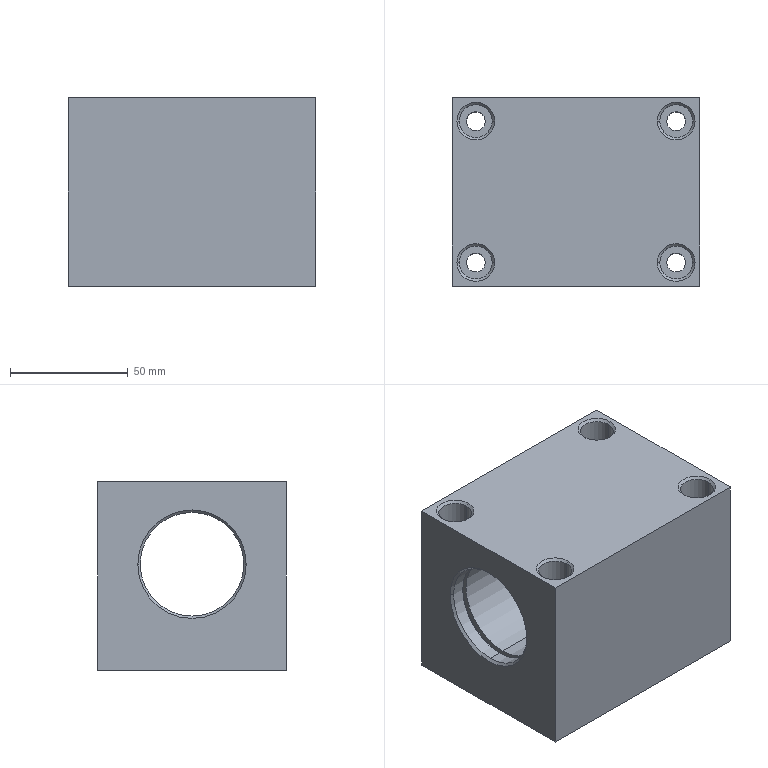Part | STEP file | Fixing block | 1 solid | 52 faces | box 105 x 80 x 80 mm | volume 486425 mm3 | cylinder 26 | plane 14 | cone 12 | commonest cylinder face diameters 8 x8 14 x8 44 x6 48.5 x4
STEP:
#1=CARTESIAN_POINT('',(-38.5,-30.,60.));
#2=VERTEX_POINT('',#1);
#3=CARTESIAN_POINT('',(-46.5,-30.,60.));
#4=VERTEX_POINT('',#3);
#5=CARTESIAN_POINT('',(-42.5,-30.,60.));
#6=DIRECTION('',(0.,0.,-1.));
#7=DIRECTION('',(-1.,0.,0.));
#8=AXIS2_PLACEMENT_3D('',#5,#6,#7);
#9=CIRCLE('',#8,4.);
#10=EDGE_CURVE('',#2,#4,#9,.T.);
#11=ORIENTED_EDGE('',*,*,#10,.F.);
#12=CARTESIAN_POINT('',(-38.5,-30.,0.));
#13=VERTEX_POINT('',#12);
#14=CARTESIAN_POINT('',(-38.5,-30.,80.));
#15=DIRECTION('',(0.,0.,-1.));
#16=VECTOR('',#15,1000.);
#17=LINE('',#14,#16);
#18=EDGE_CURVE('',#2,#13,#17,.T.);
#19=ORIENTED_EDGE('',*,*,#18,.T.);
#20=CARTESIAN_POINT('',(-46.5,-30.,0.));
#21=VERTEX_POINT('',#20);
#22=CARTESIAN_POINT('',(-42.5,-30.,0.));
#23=DIRECTION('',(0.,0.,-1.));
#24=DIRECTION('',(-1.,0.,0.));
#25=AXIS2_PLACEMENT_3D('',#22,#23,#24);
#26=CIRCLE('',#25,4.);
#27=EDGE_CURVE('',#13,#21,#26,.T.);
#28=ORIENTED_EDGE('',*,*,#27,.T.);
#29=CARTESIAN_POINT('',(-46.5,-30.,80.));
#30=DIRECTION('',(0.,0.,-1.));
#31=VECTOR('',#30,1000.);
#32=LINE('',#29,#31);
#33=EDGE_CURVE('',#4,#21,#32,.T.);
#34=ORIENTED_EDGE('',*,*,#33,.F.);
#35=EDGE_LOOP('',(#11,#19,#28,#34));
#36=FACE_OUTER_BOUND('',#35,.T.);
#37=CARTESIAN_POINT('',(-42.5,-30.,80.));
#38=DIRECTION('',(0.,0.,-1.));
#39=DIRECTION('',(-1.,0.,0.));
#40=AXIS2_PLACEMENT_3D('',#37,#38,#39);
#41=CYLINDRICAL_SURFACE('',#40,4.);
#42=ADVANCED_FACE('',(#36),#41,.F.);
#43=CARTESIAN_POINT('',(46.5,30.,60.));
#44=VERTEX_POINT('',#43);
#45=CARTESIAN_POINT('',(38.5,30.,60.));
#46=VERTEX_POINT('',#45);
#47=CARTESIAN_POINT('',(42.5,30.,60.));
#48=DIRECTION('',(0.,0.,-1.));
#49=DIRECTION('',(-1.,0.,0.));
#50=AXIS2_PLACEMENT_3D('',#47,#48,#49);
#51=CIRCLE('',#50,4.);
#52=EDGE_CURVE('',#44,#46,#51,.T.);
#53=ORIENTED_EDGE('',*,*,#52,.F.);
#54=CARTESIAN_POINT('',(46.5,30.,0.));
#55=VERTEX_POINT('',#54);
#56=CARTESIAN_POINT('',(46.5,30.,80.));
#57=DIRECTION('',(0.,0.,-1.));
#58=VECTOR('',#57,1000.);
#59=LINE('',#56,#58);
#60=EDGE_CURVE('',#44,#55,#59,.T.);
#61=ORIENTED_EDGE('',*,*,#60,.T.);
#62=CARTESIAN_POINT('',(38.5,30.,0.));
#63=VERTEX_POINT('',#62);
#64=CARTESIAN_POINT('',(42.5,30.,0.));
#65=DIRECTION('',(0.,0.,-1.));
#66=DIRECTION('',(-1.,0.,0.));
#67=AXIS2_PLACEMENT_3D('',#64,#65,#66);
#68=CIRCLE('',#67,4.);
#69=EDGE_CURVE('',#55,#63,#68,.T.);
#70=ORIENTED_EDGE('',*,*,#69,.T.);
#71=CARTESIAN_POINT('',(38.5,30.,80.));
#72=DIRECTION('',(0.,0.,-1.));
#73=VECTOR('',#72,1000.);
#74=LINE('',#71,#73);
#75=EDGE_CURVE('',#46,#63,#74,.T.);
#76=ORIENTED_EDGE('',*,*,#75,.F.);
#77=EDGE_LOOP('',(#53,#61,#70,#76));
#78=FACE_OUTER_BOUND('',#77,.T.);
#79=CARTESIAN_POINT('',(42.5,30.,80.));
#80=DIRECTION('',(0.,0.,-1.));
#81=DIRECTION('',(-1.,0.,0.));
#82=AXIS2_PLACEMENT_3D('',#79,#80,#81);
#83=CYLINDRICAL_SURFACE('',#82,4.);
#84=ADVANCED_FACE('',(#78),#83,.F.);
#85=CARTESIAN_POINT('',(-38.5,30.,60.));
#86=VERTEX_POINT('',#85);
#87=CARTESIAN_POINT('',(-46.5,30.,60.));
#88=VERTEX_POINT('',#87);
#89=CARTESIAN_POINT('',(-42.5,30.,60.));
#90=DIRECTION('',(0.,0.,-1.));
#91=DIRECTION('',(-1.,0.,0.));
#92=AXIS2_PLACEMENT_3D('',#89,#90,#91);
#93=CIRCLE('',#92,4.);
#94=EDGE_CURVE('',#86,#88,#93,.T.);
#95=ORIENTED_EDGE('',*,*,#94,.F.);
#96=CARTESIAN_POINT('',(-38.5,30.,0.));
#97=VERTEX_POINT('',#96);
#98=CARTESIAN_POINT('',(-38.5,30.,80.));
#99=DIRECTION('',(0.,0.,-1.));
#100=VECTOR('',#99,1000.);
#101=LINE('',#98,#100);
#102=EDGE_CURVE('',#86,#97,#101,.T.);
#103=ORIENTED_EDGE('',*,*,#102,.T.);
#104=CARTESIAN_POINT('',(-46.5,30.,0.));
#105=VERTEX_POINT('',#104);
#106=CARTESIAN_POINT('',(-42.5,30.,0.));
#107=DIRECTION('',(0.,0.,-1.));
#108=DIRECTION('',(-1.,0.,0.));
#109=AXIS2_PLACEMENT_3D('',#106,#107,#108);
#110=CIRCLE('',#109,4.);
#111=EDGE_CURVE('',#97,#105,#110,.T.);
#112=ORIENTED_EDGE('',*,*,#111,.T.);
#113=CARTESIAN_POINT('',(-46.5,30.,80.));
#114=DIRECTION('',(0.,0.,-1.));
#115=VECTOR('',#114,1000.);
#116=LINE('',#113,#115);
#117=EDGE_CURVE('',#88,#105,#116,.T.);
#118=ORIENTED_EDGE('',*,*,#117,.F.);
#119=EDGE_LOOP('',(#95,#103,#112,#118));
#120=FACE_OUTER_BOUND('',#119,.T.);
#121=CARTESIAN_POINT('',(-42.5,30.,80.));
#122=DIRECTION('',(0.,0.,-1.));
#123=DIRECTION('',(-1.,0.,0.));
#124=AXIS2_PLACEMENT_3D('',#121,#122,#123);
#125=CYLINDRICAL_SURFACE('',#124,4.);
#126=ADVANCED_FACE('',(#120),#125,.F.);
#127=CARTESIAN_POINT('',(46.5,-30.,60.));
#128=VERTEX_POINT('',#127);
#129=CARTESIAN_POINT('',(38.5,-30.,60.));
#130=VERTEX_POINT('',#129);
#131=CARTESIAN_POINT('',(42.5,-30.,60.));
#132=DIRECTION('',(0.,0.,-1.));
#133=DIRECTION('',(-1.,0.,0.));
#134=AXIS2_PLACEMENT_3D('',#131,#132,#133);
#135=CIRCLE('',#134,4.);
#136=EDGE_CURVE('',#128,#130,#135,.T.);
#137=ORIENTED_EDGE('',*,*,#136,.F.);
#138=CARTESIAN_POINT('',(46.5,-30.,0.));
#139=VERTEX_POINT('',#138);
#140=CARTESIAN_POINT('',(46.5,-30.,80.));
#141=DIRECTION('',(0.,0.,-1.));
#142=VECTOR('',#141,1000.);
#143=LINE('',#140,#142);
#144=EDGE_CURVE('',#128,#139,#143,.T.);
#145=ORIENTED_EDGE('',*,*,#144,.T.);
#146=CARTESIAN_POINT('',(38.5,-30.,0.));
#147=VERTEX_POINT('',#146);
#148=CARTESIAN_POINT('',(42.5,-30.,0.));
#149=DIRECTION('',(0.,0.,-1.));
#150=DIRECTION('',(-1.,0.,0.));
#151=AXIS2_PLACEMENT_3D('',#148,#149,#150);
#152=CIRCLE('',#151,4.);
#153=EDGE_CURVE('',#139,#147,#152,.T.);
#154=ORIENTED_EDGE('',*,*,#153,.T.);
#155=CARTESIAN_POINT('',(38.5,-30.,80.));
#156=DIRECTION('',(0.,0.,-1.));
#157=VECTOR('',#156,1000.);
#158=LINE('',#155,#157);
#159=EDGE_CURVE('',#130,#147,#158,.T.);
#160=ORIENTED_EDGE('',*,*,#159,.F.);
#161=EDGE_LOOP('',(#137,#145,#154,#160));
#162=FACE_OUTER_BOUND('',#161,.T.);
#163=CARTESIAN_POINT('',(42.5,-30.,80.));
#164=DIRECTION('',(0.,0.,-1.));
#165=DIRECTION('',(-1.,0.,0.));
#166=AXIS2_PLACEMENT_3D('',#163,#164,#165);
#167=CYLINDRICAL_SURFACE('',#166,4.);
#168=ADVANCED_FACE('',(#162),#167,.F.);
#169=CARTESIAN_POINT('',(-51.5,22.,45.));
#170=VERTEX_POINT('',#169);
#171=CARTESIAN_POINT('',(-51.5,0.,23.));
#172=VERTEX_POINT('',#171);
#173=CARTESIAN_POINT('',(-51.5,0.,45.));
#174=DIRECTION('',(-1.,0.,0.));
#175=DIRECTION('',(0.,0.,1.));
#176=AXIS2_PLACEMENT_3D('',#173,#174,#175);
#177=CIRCLE('',#176,22.);
#178=EDGE_CURVE('',#170,#172,#177,.T.);
#179=ORIENTED_EDGE('',*,*,#178,.F.);
#180=CARTESIAN_POINT('',(-52.5,23.,45.));
#181=VERTEX_POINT('',#180);
#182=CARTESIAN_POINT('',(-52.5,23.,45.));
#183=DIRECTION('',(-0.7071,0.7071,0.));
#184=VECTOR('',#183,1000.);
#185=LINE('',#182,#184);
#186=EDGE_CURVE('',#170,#181,#185,.T.);
#187=ORIENTED_EDGE('',*,*,#186,.T.);
#188=CARTESIAN_POINT('',(-52.5,-23.,45.));
#189=VERTEX_POINT('',#188);
#190=CARTESIAN_POINT('',(-52.5,0.,45.));
#191=DIRECTION('',(-1.,0.,0.));
#192=DIRECTION('',(0.,-1.,0.));
#193=AXIS2_PLACEMENT_3D('',#190,#191,#192);
#194=CIRCLE('',#193,23.);
#195=EDGE_CURVE('',#181,#189,#194,.T.);
#196=ORIENTED_EDGE('',*,*,#195,.T.);
#197=CARTESIAN_POINT('',(-51.5,-22.,45.));
#198=VERTEX_POINT('',#197);
#199=CARTESIAN_POINT('',(-52.5,-23.,45.));
#200=DIRECTION('',(-0.7071,-0.7071,0.));
#201=VECTOR('',#200,1000.);
#202=LINE('',#199,#201);
#203=EDGE_CURVE('',#198,#189,#202,.T.);
#204=ORIENTED_EDGE('',*,*,#203,.F.);
#205=CARTESIAN_POINT('',(-51.5,0.,45.));
#206=DIRECTION('',(-1.,0.,0.));
#207=DIRECTION('',(0.,0.,1.));
#208=AXIS2_PLACEMENT_3D('',#205,#206,#207);
#209=CIRCLE('',#208,22.);
#210=EDGE_CURVE('',#172,#198,#209,.T.);
#211=ORIENTED_EDGE('',*,*,#210,.F.);
#212=EDGE_LOOP('',(#179,#187,#196,#204,#211));
#213=FACE_OUTER_BOUND('',#212,.T.);
#214=CARTESIAN_POINT('',(-52.5,0.,45.));
#215=DIRECTION('',(-1.,0.,0.));
#216=DIRECTION('',(0.,-1.,0.));
#217=AXIS2_PLACEMENT_3D('',#214,#215,#216);
#218=CONICAL_SURFACE('',#217,23.,0.7854);
#219=ADVANCED_FACE('',(#213),#218,.F.);
#220=CARTESIAN_POINT('',(-49.5,30.,79.));
#221=VERTEX_POINT('',#220);
#222=CARTESIAN_POINT('',(-35.5,30.,79.));
#223=VERTEX_POINT('',#222);
#224=CARTESIAN_POINT('',(-42.5,30.,79.));
#225=DIRECTION('',(0.,0.,1.));
#226=DIRECTION('',(1.,0.,0.));
#227=AXIS2_PLACEMENT_3D('',#224,#225,#226);
#228=CIRCLE('',#227,7.);
#229=EDGE_CURVE('',#221,#223,#228,.T.);
#230=ORIENTED_EDGE('',*,*,#229,.F.);
#231=CARTESIAN_POINT('',(-50.5,30.,80.));
#232=VERTEX_POINT('',#231);
#233=CARTESIAN_POINT('',(-50.5,30.,80.));
#234=DIRECTION('',(-0.7071,0.,0.7071));
#235=VECTOR('',#234,1000.);
#236=LINE('',#233,#235);
#237=EDGE_CURVE('',#221,#232,#236,.T.);
#238=ORIENTED_EDGE('',*,*,#237,.T.);
#239=CARTESIAN_POINT('',(-34.5,30.,80.));
#240=VERTEX_POINT('',#239);
#241=CARTESIAN_POINT('',(-42.5,30.,80.));
#242=DIRECTION('',(0.,0.,-1.));
#243=DIRECTION('',(1.,0.,0.));
#244=AXIS2_PLACEMENT_3D('',#241,#242,#243);
#245=CIRCLE('',#244,8.);
#246=EDGE_CURVE('',#240,#232,#245,.T.);
#247=ORIENTED_EDGE('',*,*,#246,.F.);
#248=CARTESIAN_POINT('',(-34.5,30.,80.));
#249=DIRECTION('',(0.7071,0.,0.7071));
#250=VECTOR('',#249,1000.);
#251=LINE('',#248,#250);
#252=EDGE_CURVE('',#223,#240,#251,.T.);
#253=ORIENTED_EDGE('',*,*,#252,.F.);
#254=EDGE_LOOP('',(#230,#238,#247,#253));
#255=FACE_OUTER_BOUND('',#254,.T.);
#256=CARTESIAN_POINT('',(-42.5,30.,80.));
#257=DIRECTION('',(0.,0.,1.));
#258=DIRECTION('',(1.,0.,0.));
#259=AXIS2_PLACEMENT_3D('',#256,#257,#258);
#260=CONICAL_SURFACE('',#259,8.,0.7854);
#261=ADVANCED_FACE('',(#255),#260,.F.);
#262=CARTESIAN_POINT('',(-49.5,-30.,79.));
#263=VERTEX_POINT('',#262);
#264=CARTESIAN_POINT('',(-35.5,-30.,79.));
#265=VERTEX_POINT('',#264);
#266=CARTESIAN_POINT('',(-42.5,-30.,79.));
#267=DIRECTION('',(0.,0.,1.));
#268=DIRECTION('',(1.,0.,0.));
#269=AXIS2_PLACEMENT_3D('',#266,#267,#268);
#270=CIRCLE('',#269,7.);
#271=EDGE_CURVE('',#263,#265,#270,.T.);
#272=ORIENTED_EDGE('',*,*,#271,.F.);
#273=CARTESIAN_POINT('',(-50.5,-30.,80.));
#274=VERTEX_POINT('',#273);
#275=CARTESIAN_POINT('',(-50.5,-30.,80.));
#276=DIRECTION('',(-0.7071,0.,0.7071));
#277=VECTOR('',#276,1000.);
#278=LINE('',#275,#277);
#279=EDGE_CURVE('',#263,#274,#278,.T.);
#280=ORIENTED_EDGE('',*,*,#279,.T.);
#281=CARTESIAN_POINT('',(-34.5,-30.,80.));
#282=VERTEX_POINT('',#281);
#283=CARTESIAN_POINT('',(-42.5,-30.,80.));
#284=DIRECTION('',(0.,0.,-1.));
#285=DIRECTION('',(1.,0.,0.));
#286=AXIS2_PLACEMENT_3D('',#283,#284,#285);
#287=CIRCLE('',#286,8.);
#288=EDGE_CURVE('',#282,#274,#287,.T.);
#289=ORIENTED_EDGE('',*,*,#288,.F.);
#290=CARTESIAN_POINT('',(-34.5,-30.,80.));
#291=DIRECTION('',(0.7071,0.,0.7071));
#292=VECTOR('',#291,1000.);
#293=LINE('',#290,#292);
#294=EDGE_CURVE('',#265,#282,#293,.T.);
#295=ORIENTED_EDGE('',*,*,#294,.F.);
#296=EDGE_LOOP('',(#272,#280,#289,#295));
#297=FACE_OUTER_BOUND('',#296,.T.);
#298=CARTESIAN_POINT('',(-42.5,-30.,80.));
#299=DIRECTION('',(0.,0.,1.));
#300=DIRECTION('',(1.,0.,0.));
#301=AXIS2_PLACEMENT_3D('',#298,#299,#300);
#302=CONICAL_SURFACE('',#301,8.,0.7854);
#303=ADVANCED_FACE('',(#297),#302,.F.);
#304=CARTESIAN_POINT('',(35.5,30.,79.));
#305=VERTEX_POINT('',#304);
#306=CARTESIAN_POINT('',(49.5,30.,79.));
#307=VERTEX_POINT('',#306);
#308=CARTESIAN_POINT('',(42.5,30.,79.));
#309=DIRECTION('',(0.,0.,1.));
#310=DIRECTION('',(1.,0.,0.));
#311=AXIS2_PLACEMENT_3D('',#308,#309,#310);
#312=CIRCLE('',#311,7.);
#313=EDGE_CURVE('',#305,#307,#312,.T.);
#314=ORIENTED_EDGE('',*,*,#313,.F.);
#315=CARTESIAN_POINT('',(34.5,30.,80.));
#316=VERTEX_POINT('',#315);
#317=CARTESIAN_POINT('',(34.5,30.,80.));
#318=DIRECTION('',(-0.7071,0.,0.7071));
#319=VECTOR('',#318,1000.);
#320=LINE('',#317,#319);
#321=EDGE_CURVE('',#305,#316,#320,.T.);
#322=ORIENTED_EDGE('',*,*,#321,.T.);
#323=CARTESIAN_POINT('',(50.5,30.,80.));
#324=VERTEX_POINT('',#323);
#325=CARTESIAN_POINT('',(42.5,30.,80.));
#326=DIRECTION('',(0.,0.,-1.));
#327=DIRECTION('',(1.,0.,0.));
#328=AXIS2_PLACEMENT_3D('',#325,#326,#327);
#329=CIRCLE('',#328,8.);
#330=EDGE_CURVE('',#324,#316,#329,.T.);
#331=ORIENTED_EDGE('',*,*,#330,.F.);
#332=CARTESIAN_POINT('',(50.5,30.,80.));
#333=DIRECTION('',(0.7071,0.,0.7071));
#334=VECTOR('',#333,1000.);
#335=LINE('',#332,#334);
#336=EDGE_CURVE('',#307,#324,#335,.T.);
#337=ORIENTED_EDGE('',*,*,#336,.F.);
#338=EDGE_LOOP('',(#314,#322,#331,#337));
#339=FACE_OUTER_BOUND('',#338,.T.);
#340=CARTESIAN_POINT('',(42.5,30.,80.));
#341=DIRECTION('',(0.,0.,1.));
#342=DIRECTION('',(1.,0.,0.));
#343=AXIS2_PLACEMENT_3D('',#340,#341,#342);
#344=CONICAL_SURFACE('',#343,8.,0.7854);
#345=ADVANCED_FACE('',(#339),#344,.F.);
#346=CARTESIAN_POINT('',(35.5,-30.,79.));
#347=VERTEX_POINT('',#346);
#348=CARTESIAN_POINT('',(49.5,-30.,79.));
#349=VERTEX_POINT('',#348);
#350=CARTESIAN_POINT('',(42.5,-30.,79.));
#351=DIRECTION('',(0.,0.,1.));
#352=DIRECTION('',(1.,0.,0.));
#353=AXIS2_PLACEMENT_3D('',#350,#351,#352);
#354=CIRCLE('',#353,7.);
#355=EDGE_CURVE('',#347,#349,#354,.T.);
#356=ORIENTED_EDGE('',*,*,#355,.F.);
#357=CARTESIAN_POINT('',(34.5,-30.,80.));
#358=VERTEX_POINT('',#357);
#359=CARTESIAN_POINT('',(34.5,-30.,80.));
#360=DIRECTION('',(-0.7071,0.,0.7071));
#361=VECTOR('',#360,1000.);
#362=LINE('',#359,#361);
#363=EDGE_CURVE('',#347,#358,#362,.T.);
#364=ORIENTED_EDGE('',*,*,#363,.T.);
#365=CARTESIAN_POINT('',(50.5,-30.,80.));
#366=VERTEX_POINT('',#365);
#367=CARTESIAN_POINT('',(42.5,-30.,80.));
#368=DIRECTION('',(0.,0.,-1.));
#369=DIRECTION('',(1.,0.,0.));
#370=AXIS2_PLACEMENT_3D('',#367,#368,#369);
#371=CIRCLE('',#370,8.);
#372=EDGE_CURVE('',#366,#358,#371,.T.);
#373=ORIENTED_EDGE('',*,*,#372,.F.);
#374=CARTESIAN_POINT('',(50.5,-30.,80.));
#375=DIRECTION('',(0.7071,0.,0.7071));
#376=VECTOR('',#375,1000.);
#377=LINE('',#374,#376);
#378=EDGE_CURVE('',#349,#366,#377,.T.);
#379=ORIENTED_EDGE('',*,*,#378,.F.);
#380=EDGE_LOOP('',(#356,#364,#373,#379));
#381=FACE_OUTER_BOUND('',#380,.T.);
#382=CARTESIAN_POINT('',(42.5,-30.,80.));
#383=DIRECTION('',(0.,0.,1.));
#384=DIRECTION('',(1.,0.,0.));
#385=AXIS2_PLACEMENT_3D('',#382,#383,#384);
#386=CONICAL_SURFACE('',#385,8.,0.7854);
#387=ADVANCED_FACE('',(#381),#386,.F.);
#388=CARTESIAN_POINT('',(51.5,-22.,45.));
#389=VERTEX_POINT('',#388);
#390=CARTESIAN_POINT('',(51.5,0.,23.));
#391=VERTEX_POINT('',#390);
#392=CARTESIAN_POINT('',(51.5,0.,45.));
#393=DIRECTION('',(1.,0.,0.));
#394=DIRECTION('',(0.,0.,-1.));
#395=AXIS2_PLACEMENT_3D('',#392,#393,#394);
#396=CIRCLE('',#395,22.);
#397=EDGE_CURVE('',#389,#391,#396,.T.);
#398=ORIENTED_EDGE('',*,*,#397,.F.);
#399=CARTESIAN_POINT('',(52.5,-23.,45.));
#400=VERTEX_POINT('',#399);
#401=CARTESIAN_POINT('',(52.5,-23.,45.));
#402=DIRECTION('',(0.7071,-0.7071,0.));
#403=VECTOR('',#402,1000.);
#404=LINE('',#401,#403);
#405=EDGE_CURVE('',#389,#400,#404,.T.);
#406=ORIENTED_EDGE('',*,*,#405,.T.);
#407=CARTESIAN_POINT('',(52.5,23.,45.));
#408=VERTEX_POINT('',#407);
#409=CARTESIAN_POINT('',(52.5,0.,45.));
#410=DIRECTION('',(1.,0.,0.));
#411=DIRECTION('',(0.,1.,0.));
#412=AXIS2_PLACEMENT_3D('',#409,#410,#411);
#413=CIRCLE('',#412,23.);
#414=EDGE_CURVE('',#400,#408,#413,.T.);
#415=ORIENTED_EDGE('',*,*,#414,.T.);
#416=CARTESIAN_POINT('',(51.5,22.,45.));
#417=VERTEX_POINT('',#416);
#418=CARTESIAN_POINT('',(52.5,23.,45.));
#419=DIRECTION('',(0.7071,0.7071,0.));
#420=VECTOR('',#419,1000.);
#421=LINE('',#418,#420);
#422=EDGE_CURVE('',#417,#408,#421,.T.);
#423=ORIENTED_EDGE('',*,*,#422,.F.);
#424=CARTESIAN_POINT('',(51.5,0.,45.));
#425=DIRECTION('',(1.,0.,0.));
#426=DIRECTION('',(0.,0.,-1.));
#427=AXIS2_PLACEMENT_3D('',#424,#425,#426);
#428=CIRCLE('',#427,22.);
#429=EDGE_CURVE('',#391,#417,#428,.T.);
#430=ORIENTED_EDGE('',*,*,#429,.F.);
#431=EDGE_LOOP('',(#398,#406,#415,#423,#430));
#432=FACE_OUTER_BOUND('',#431,.T.);
#433=CARTESIAN_POINT('',(52.5,0.,45.));
#434=DIRECTION('',(1.,0.,0.));
#435=DIRECTION('',(0.,1.,0.));
#436=AXIS2_PLACEMENT_3D('',#433,#434,#435);
#437=CONICAL_SURFACE('',#436,23.,0.7854);
#438=ADVANCED_FACE('',(#432),#437,.F.);
#439=CARTESIAN_POINT('',(-46.,0.,23.));
#440=VERTEX_POINT('',#439);
#441=CARTESIAN_POINT('',(-46.,0.,67.));
#442=VERTEX_POINT('',#441);
#443=CARTESIAN_POINT('',(-46.,0.,45.));
#444=DIRECTION('',(-1.,0.,0.));
#445=DIRECTION('',(0.,0.,1.));
#446=AXIS2_PLACEMENT_3D('',#443,#444,#445);
#447=CIRCLE('',#446,22.);
#448=EDGE_CURVE('',#440,#442,#447,.T.);
#449=ORIENTED_EDGE('',*,*,#448,.F.);
#450=CARTESIAN_POINT('',(52.5,0.,23.));
#451=DIRECTION('',(-1.,0.,0.));
#452=VECTOR('',#451,1000.);
#453=LINE('',#450,#452);
#454=EDGE_CURVE('',#440,#172,#453,.T.);
#455=ORIENTED_EDGE('',*,*,#454,.T.);
#456=ORIENTED_EDGE('',*,*,#210,.T.);
#457=CARTESIAN_POINT('',(-51.5,0.,67.));
#458=VERTEX_POINT('',#457);
#459=CARTESIAN_POINT('',(-51.5,0.,45.));
#460=DIRECTION('',(-1.,0.,0.));
#461=DIRECTION('',(0.,0.,1.));
#462=AXIS2_PLACEMENT_3D('',#459,#460,#461);
#463=CIRCLE('',#462,22.);
#464=EDGE_CURVE('',#198,#458,#463,.T.);
#465=ORIENTED_EDGE('',*,*,#464,.T.);
#466=CARTESIAN_POINT('',(52.5,0.,67.));
#467=DIRECTION('',(-1.,0.,0.));
#468=VECTOR('',#467,1000.);
#469=LINE('',#466,#468);
#470=EDGE_CURVE('',#442,#458,#469,.T.);
#471=ORIENTED_EDGE('',*,*,#470,.F.);
#472=EDGE_LOOP('',(#449,#455,#456,#465,#471));
#473=FACE_OUTER_BOUND('',#472,.T.);
#474=CARTESIAN_POINT('',(52.5,0.,45.));
#475=DIRECTION('',(-1.,0.,0.));
#476=DIRECTION('',(0.,0.,1.));
#477=AXIS2_PLACEMENT_3D('',#474,#475,#476);
#478=CYLINDRICAL_SURFACE('',#477,22.);
#479=ADVANCED_FACE('',(#473),#478,.F.);
#480=CARTESIAN_POINT('',(-49.5,30.,60.));
#481=VERTEX_POINT('',#480);
#482=CARTESIAN_POINT('',(-35.5,30.,60.));
#483=VERTEX_POINT('',#482);
#484=CARTESIAN_POINT('',(-42.5,30.,60.));
#485=DIRECTION('',(0.,0.,1.));
#486=DIRECTION('',(1.,0.,0.));
#487=AXIS2_PLACEMENT_3D('',#484,#485,#486);
#488=CIRCLE('',#487,7.);
#489=EDGE_CURVE('',#481,#483,#488,.T.);
#490=ORIENTED_EDGE('',*,*,#489,.F.);
#491=CARTESIAN_POINT('',(-49.5,30.,60.));
#492=DIRECTION('',(0.,0.,1.));
#493=VECTOR('',#492,1000.);
#494=LINE('',#491,#493);
#495=EDGE_CURVE('',#481,#221,#494,.T.);
#496=ORIENTED_EDGE('',*,*,#495,.T.);
#497=ORIENTED_EDGE('',*,*,#229,.T.);
#498=CARTESIAN_POINT('',(-35.5,30.,60.));
#499=DIRECTION('',(0.,0.,1.));
#500=VECTOR('',#499,1000.);
#501=LINE('',#498,#500);
#502=EDGE_CURVE('',#483,#223,#501,.T.);
#503=ORIENTED_EDGE('',*,*,#502,.F.);
#504=EDGE_LOOP('',(#490,#496,#497,#503));
#505=FACE_OUTER_BOUND('',#504,.T.);
#506=CARTESIAN_POINT('',(-42.5,30.,60.));
#507=DIRECTION('',(0.,0.,1.));
#508=DIRECTION('',(1.,0.,0.));
#509=AXIS2_PLACEMENT_3D('',#506,#507,#508);
#510=CYLINDRICAL_SURFACE('',#509,7.);
#511=ADVANCED_FACE('',(#505),#510,.F.);
#512=CARTESIAN_POINT('',(-49.5,-30.,60.));
#513=VERTEX_POINT('',#512);
#514=CARTESIAN_POINT('',(-35.5,-30.,60.));
#515=VERTEX_POINT('',#514);
#516=CARTESIAN_POINT('',(-42.5,-30.,60.));
#517=DIRECTION('',(0.,0.,1.));
#518=DIRECTION('',(1.,0.,0.));
#519=AXIS2_PLACEMENT_3D('',#516,#517,#518);
#520=CIRCLE('',#519,7.);
#521=EDGE_CURVE('',#513,#515,#520,.T.);
#522=ORIENTED_EDGE('',*,*,#521,.F.);
#523=CARTESIAN_POINT('',(-49.5,-30.,60.));
#524=DIRECTION('',(0.,0.,1.));
#525=VECTOR('',#524,1000.);
#526=LINE('',#523,#525);
#527=EDGE_CURVE('',#513,#263,#526,.T.);
#528=ORIENTED_EDGE('',*,*,#527,.T.);
#529=ORIENTED_EDGE('',*,*,#271,.T.);
#530=CARTESIAN_POINT('',(-35.5,-30.,60.));
#531=DIRECTION('',(0.,0.,1.));
#532=VECTOR('',#531,1000.);
#533=LINE('',#530,#532);
#534=EDGE_CURVE('',#515,#265,#533,.T.);
#535=ORIENTED_EDGE('',*,*,#534,.F.);
#536=EDGE_LOOP('',(#522,#528,#529,#535));
#537=FACE_OUTER_BOUND('',#536,.T.);
#538=CARTESIAN_POINT('',(-42.5,-30.,60.));
#539=DIRECTION('',(0.,0.,1.));
#540=DIRECTION('',(1.,0.,0.));
#541=AXIS2_PLACEMENT_3D('',#538,#539,#540);
#542=CYLINDRICAL_SURFACE('',#541,7.);
#543=ADVANCED_FACE('',(#537),#542,.F.);
#544=CARTESIAN_POINT('',(35.5,30.,60.));
#545=VERTEX_POINT('',#544);
#546=CARTESIAN_POINT('',(49.5,30.,60.));
#547=VERTEX_POINT('',#546);
#548=CARTESIAN_POINT('',(42.5,30.,60.));
#549=DIRECTION('',(0.,0.,1.));
#550=DIRECTION('',(1.,0.,0.));
#551=AXIS2_PLACEMENT_3D('',#548,#549,#550);
#552=CIRCLE('',#551,7.);
#553=EDGE_CURVE('',#545,#547,#552,.T.);
#554=ORIENTED_EDGE('',*,*,#553,.F.);
#555=CARTESIAN_POINT('',(35.5,30.,60.));
#556=DIRECTION('',(0.,0.,1.));
#557=VECTOR('',#556,1000.);
#558=LINE('',#555,#557);
#559=EDGE_CURVE('',#545,#305,#558,.T.);
#560=ORIENTED_EDGE('',*,*,#559,.T.);
#561=ORIENTED_EDGE('',*,*,#313,.T.);
#562=CARTESIAN_POINT('',(49.5,30.,60.));
#563=DIRECTION('',(0.,0.,1.));
#564=VECTOR('',#563,1000.);
#565=LINE('',#562,#564);
#566=EDGE_CURVE('',#547,#307,#565,.T.);
#567=ORIENTED_EDGE('',*,*,#566,.F.);
#568=EDGE_LOOP('',(#554,#560,#561,#567));
#569=FACE_OUTER_BOUND('',#568,.T.);
#570=CARTESIAN_POINT('',(42.5,30.,60.));
#571=DIRECTION('',(0.,0.,1.));
#572=DIRECTION('',(1.,0.,0.));
#573=AXIS2_PLACEMENT_3D('',#570,#571,#572);
#574=CYLINDRICAL_SURFACE('',#573,7.);
#575=ADVANCED_FACE('',(#569),#574,.F.);
#576=CARTESIAN_POINT('',(35.5,-30.,60.));
#577=VERTEX_POINT('',#576);
#578=CARTESIAN_POINT('',(49.5,-30.,60.));
#579=VERTEX_POINT('',#578);
#580=CARTESIAN_POINT('',(42.5,-30.,60.));
#581=DIRECTION('',(0.,0.,1.));
#582=DIRECTION('',(1.,0.,0.));
#583=AXIS2_PLACEMENT_3D('',#580,#581,#582);
#584=CIRCLE('',#583,7.);
#585=EDGE_CURVE('',#577,#579,#584,.T.);
#586=ORIENTED_EDGE('',*,*,#585,.F.);
#587=CARTESIAN_POINT('',(35.5,-30.,60.));
#588=DIRECTION('',(0.,0.,1.));
#589=VECTOR('',#588,1000.);
#590=LINE('',#587,#589);
#591=EDGE_CURVE('',#577,#347,#590,.T.);
#592=ORIENTED_EDGE('',*,*,#591,.T.);
#593=ORIENTED_EDGE('',*,*,#355,.T.);
#594=CARTESIAN_POINT('',(49.5,-30.,60.));
#595=DIRECTION('',(0.,0.,1.));
#596=VECTOR('',#595,1000.);
#597=LINE('',#594,#596);
#598=EDGE_CURVE('',#579,#349,#597,.T.);
#599=ORIENTED_EDGE('',*,*,#598,.F.);
#600=EDGE_LOOP('',(#586,#592,#593,#599));
#601=FACE_OUTER_BOUND('',#600,.T.);
#602=CARTESIAN_POINT('',(42.5,-30.,60.));
#603=DIRECTION('',(0.,0.,1.));
#604=DIRECTION('',(1.,0.,0.));
#605=AXIS2_PLACEMENT_3D('',#602,#603,#604);
#606=CYLINDRICAL_SURFACE('',#605,7.);
#607=ADVANCED_FACE('',(#601),#606,.F.);
#608=CARTESIAN_POINT('',(51.5,0.,67.));
#609=VERTEX_POINT('',#608);
#610=CARTESIAN_POINT('',(51.5,0.,45.));
#611=DIRECTION('',(1.,0.,0.));
#612=DIRECTION('',(0.,0.,-1.));
#613=AXIS2_PLACEMENT_3D('',#610,#611,#612);
#614=CIRCLE('',#613,22.);
#615=EDGE_CURVE('',#609,#389,#614,.T.);
#616=ORIENTED_EDGE('',*,*,#615,.T.);
#617=ORIENTED_EDGE('',*,*,#397,.T.);
#618=CARTESIAN_POINT('',(46.,0.,23.));
#619=VERTEX_POINT('',#618);
#620=CARTESIAN_POINT('',(52.5,0.,23.));
#621=DIRECTION('',(-1.,0.,0.));
#622=VECTOR('',#621,1000.);
#623=LINE('',#620,#622);
#624=EDGE_CURVE('',#391,#619,#623,.T.);
#625=ORIENTED_EDGE('',*,*,#624,.T.);
#626=CARTESIAN_POINT('',(46.,0.,67.));
#627=VERTEX_POINT('',#626);
#628=CARTESIAN_POINT('',(46.,0.,45.));
#629=DIRECTION('',(1.,0.,0.));
#630=DIRECTION('',(0.,0.,1.));
#631=AXIS2_PLACEMENT_3D('',#628,#629,#630);
#632=CIRCLE('',#631,22.);
#633=EDGE_CURVE('',#627,#619,#632,.T.);
#634=ORIENTED_EDGE('',*,*,#633,.F.);
#635=CARTESIAN_POINT('',(52.5,0.,67.));
#636=DIRECTION('',(-1.,0.,0.));
#637=VECTOR('',#636,1000.);
#638=LINE('',#635,#637);
#639=EDGE_CURVE('',#609,#627,#638,.T.);
#640=ORIENTED_EDGE('',*,*,#639,.F.);
#641=EDGE_LOOP('',(#616,#617,#625,#634,#640));
#642=FACE_OUTER_BOUND('',#641,.T.);
#643=CARTESIAN_POINT('',(52.5,0.,45.));
#644=DIRECTION('',(-1.,0.,0.));
#645=DIRECTION('',(0.,0.,1.));
#646=AXIS2_PLACEMENT_3D('',#643,#644,#645);
#647=CYLINDRICAL_SURFACE('',#646,22.);
#648=ADVANCED_FACE('',(#642),#647,.F.);
#649=CARTESIAN_POINT('',(-46.,0.,69.25));
#650=VERTEX_POINT('',#649);
#651=CARTESIAN_POINT('',(-46.,0.,20.75));
#652=VERTEX_POINT('',#651);
#653=CARTESIAN_POINT('',(-46.,0.,45.));
#654=DIRECTION('',(1.,0.,0.));
#655=DIRECTION('',(0.,0.,-1.));
#656=AXIS2_PLACEMENT_3D('',#653,#654,#655);
#657=CIRCLE('',#656,24.25);
#658=EDGE_CURVE('',#650,#652,#657,.T.);
#659=ORIENTED_EDGE('',*,*,#658,.F.);
#660=CARTESIAN_POINT('',(-44.,0.,69.25));
#661=VERTEX_POINT('',#660);
#662=CARTESIAN_POINT('',(5.937,0.,69.25));
#663=DIRECTION('',(1.,0.,0.));
#664=VECTOR('',#663,1000.);
#665=LINE('',#662,#664);
#666=EDGE_CURVE('',#650,#661,#665,.T.);
#667=ORIENTED_EDGE('',*,*,#666,.T.);
#668=CARTESIAN_POINT('',(-44.,0.,20.75));
#669=VERTEX_POINT('',#668);
#670=CARTESIAN_POINT('',(-44.,0.,45.));
#671=DIRECTION('',(-1.,0.,0.));
#672=DIRECTION('',(0.,0.,-1.));
#673=AXIS2_PLACEMENT_3D('',#670,#671,#672);
#674=CIRCLE('',#673,24.25);
#675=EDGE_CURVE('',#669,#661,#674,.T.);
#676=ORIENTED_EDGE('',*,*,#675,.F.);
#677=CARTESIAN_POINT('',(5.937,0.,20.75));
#678=DIRECTION('',(1.,0.,0.));
#679=VECTOR('',#678,1000.);
#680=LINE('',#677,#679);
#681=EDGE_CURVE('',#652,#669,#680,.T.);
#682=ORIENTED_EDGE('',*,*,#681,.F.);
#683=EDGE_LOOP('',(#659,#667,#676,#682));
#684=FACE_OUTER_BOUND('',#683,.T.);
#685=CARTESIAN_POINT('',(5.937,0.,45.));
#686=DIRECTION('',(1.,0.,0.));
#687=DIRECTION('',(0.,0.,-1.));
#688=AXIS2_PLACEMENT_3D('',#685,#686,#687);
#689=CYLINDRICAL_SURFACE('',#688,24.25);
#690=ADVANCED_FACE('',(#684),#689,.F.);
#691=CARTESIAN_POINT('',(46.,0.,69.25));
#692=VERTEX_POINT('',#691);
#693=CARTESIAN_POINT('',(46.,0.,20.75));
#694=VERTEX_POINT('',#693);
#695=CARTESIAN_POINT('',(46.,0.,45.));
#696=DIRECTION('',(1.,0.,0.));
#697=DIRECTION('',(0.,0.,1.));
#698=AXIS2_PLACEMENT_3D('',#695,#696,#697);
#699=CIRCLE('',#698,24.25);
#700=EDGE_CURVE('',#692,#694,#699,.T.);
#701=ORIENTED_EDGE('',*,*,#700,.T.);
#702=CARTESIAN_POINT('',(44.,0.,20.75));
#703=VERTEX_POINT('',#702);
#704=CARTESIAN_POINT('',(8.882,0.,20.75));
#705=DIRECTION('',(-1.,0.,0.));
#706=VECTOR('',#705,1000.);
#707=LINE('',#704,#706);
#708=EDGE_CURVE('',#694,#703,#707,.T.);
#709=ORIENTED_EDGE('',*,*,#708,.T.);
#710=CARTESIAN_POINT('',(44.,0.,69.25));
#711=VERTEX_POINT('',#710);
#712=CARTESIAN_POINT('',(44.,0.,45.));
#713=DIRECTION('',(1.,0.,0.));
#714=DIRECTION('',(0.,0.,1.));
#715=AXIS2_PLACEMENT_3D('',#712,#713,#714);
#716=CIRCLE('',#715,24.25);
#717=EDGE_CURVE('',#711,#703,#716,.T.);
#718=ORIENTED_EDGE('',*,*,#717,.F.);
#719=CARTESIAN_POINT('',(8.882,0.,69.25));
#720=DIRECTION('',(-1.,0.,0.));
#721=VECTOR('',#720,1000.);
#722=LINE('',#719,#721);
#723=EDGE_CURVE('',#692,#711,#722,.T.);
#724=ORIENTED_EDGE('',*,*,#723,.F.);
#725=EDGE_LOOP('',(#701,#709,#718,#724));
#726=FACE_OUTER_BOUND('',#725,.T.);
#727=CARTESIAN_POINT('',(8.882,0.,45.));
#728=DIRECTION('',(-1.,0.,0.));
#729=DIRECTION('',(0.,0.,1.));
#730=AXIS2_PLACEMENT_3D('',#727,#728,#729);
#731=CYLINDRICAL_SURFACE('',#730,24.25);
#732=ADVANCED_FACE('',(#726),#731,.F.);
#733=CARTESIAN_POINT('',(44.,0.,67.));
#734=VERTEX_POINT('',#733);
#735=CARTESIAN_POINT('',(44.,0.,23.));
#736=VERTEX_POINT('',#735);
#737=CARTESIAN_POINT('',(44.,0.,45.));
#738=DIRECTION('',(1.,0.,0.));
#739=DIRECTION('',(0.,0.,1.));
#740=AXIS2_PLACEMENT_3D('',#737,#738,#739);
#741=CIRCLE('',#740,22.);
#742=EDGE_CURVE('',#734,#736,#741,.T.);
#743=ORIENTED_EDGE('',*,*,#742,.T.);
#744=CARTESIAN_POINT('',(-44.,0.,23.));
#745=VERTEX_POINT('',#744);
#746=CARTESIAN_POINT('',(52.5,0.,23.));
#747=DIRECTION('',(-1.,0.,0.));
#748=VECTOR('',#747,1000.);
#749=LINE('',#746,#748);
#750=EDGE_CURVE('',#736,#745,#749,.T.);
#751=ORIENTED_EDGE('',*,*,#750,.T.);
#752=CARTESIAN_POINT('',(-44.,0.,67.));
#753=VERTEX_POINT('',#752);
#754=CARTESIAN_POINT('',(-44.,0.,45.));
#755=DIRECTION('',(1.,0.,0.));
#756=DIRECTION('',(0.,0.,1.));
#757=AXIS2_PLACEMENT_3D('',#754,#755,#756);
#758=CIRCLE('',#757,22.);
#759=EDGE_CURVE('',#753,#745,#758,.T.);
#760=ORIENTED_EDGE('',*,*,#759,.F.);
#761=CARTESIAN_POINT('',(52.5,0.,67.));
#762=DIRECTION('',(-1.,0.,0.));
#763=VECTOR('',#762,1000.);
#764=LINE('',#761,#763);
#765=EDGE_CURVE('',#734,#753,#764,.T.);
#766=ORIENTED_EDGE('',*,*,#765,.F.);
#767=EDGE_LOOP('',(#743,#751,#760,#766));
#768=FACE_OUTER_BOUND('',#767,.T.);
#769=CARTESIAN_POINT('',(52.5,0.,45.));
#770=DIRECTION('',(-1.,0.,0.));
#771=DIRECTION('',(0.,0.,1.));
#772=AXIS2_PLACEMENT_3D('',#769,#770,#771);
#773=CYLINDRICAL_SURFACE('',#772,22.);
#774=ADVANCED_FACE('',(#768),#773,.F.);
#775=CARTESIAN_POINT('',(-52.5,40.,80.));
#776=VERTEX_POINT('',#775);
#777=CARTESIAN_POINT('',(-52.5,40.,0.));
#778=VERTEX_POINT('',#777);
#779=CARTESIAN_POINT('',(-52.5,40.,80.));
#780=DIRECTION('',(0.,0.,-1.));
#781=VECTOR('',#780,1000.);
#782=LINE('',#779,#781);
#783=EDGE_CURVE('',#776,#778,#782,.T.);
#784=ORIENTED_EDGE('',*,*,#783,.F.);
#785=CARTESIAN_POINT('',(52.5,40.,80.));
#786=VERTEX_POINT('',#785);
#787=CARTESIAN_POINT('',(-52.5,40.,80.));
#788=DIRECTION('',(-1.,0.,0.));
#789=VECTOR('',#788,1000.);
#790=LINE('',#787,#789);
#791=EDGE_CURVE('',#786,#776,#790,.T.);
#792=ORIENTED_EDGE('',*,*,#791,.F.);
#793=CARTESIAN_POINT('',(52.5,40.,0.));
#794=VERTEX_POINT('',#793);
#795=CARTESIAN_POINT('',(52.5,40.,80.));
#796=DIRECTION('',(0.,0.,1.));
#797=VECTOR('',#796,1000.);
#798=LINE('',#795,#797);
#799=EDGE_CURVE('',#794,#786,#798,.T.);
#800=ORIENTED_EDGE('',*,*,#799,.F.);
#801=CARTESIAN_POINT('',(-52.5,40.,0.));
#802=DIRECTION('',(1.,0.,0.));
#803=VECTOR('',#802,1000.);
#804=LINE('',#801,#803);
#805=EDGE_CURVE('',#778,#794,#804,.T.);
#806=ORIENTED_EDGE('',*,*,#805,.F.);
#807=EDGE_LOOP('',(#784,#792,#800,#806));
#808=FACE_OUTER_BOUND('',#807,.T.);
#809=CARTESIAN_POINT('',(-52.5,40.,80.));
#810=DIRECTION('',(0.,-1.,0.));
#811=DIRECTION('',(0.,0.,-1.));
#812=AXIS2_PLACEMENT_3D('',#809,#810,#811);
#813=PLANE('',#812);
#814=ADVANCED_FACE('',(#808),#813,.F.);
#815=CARTESIAN_POINT('',(-42.5,-30.,0.));
#816=DIRECTION('',(0.,0.,-1.));
#817=DIRECTION('',(-1.,0.,0.));
#818=AXIS2_PLACEMENT_3D('',#815,#816,#817);
#819=CIRCLE('',#818,4.);
#820=EDGE_CURVE('',#21,#13,#819,.T.);
#821=ORIENTED_EDGE('',*,*,#820,.F.);
#822=ORIENTED_EDGE('',*,*,#27,.F.);
#823=EDGE_LOOP('',(#821,#822));
#824=FACE_BOUND('',#823,.T.);
#825=CARTESIAN_POINT('',(42.5,30.,0.));
#826=DIRECTION('',(0.,0.,-1.));
#827=DIRECTION('',(-1.,0.,0.));
#828=AXIS2_PLACEMENT_3D('',#825,#826,#827);
#829=CIRCLE('',#828,4.);
#830=EDGE_CURVE('',#63,#55,#829,.T.);
#831=ORIENTED_EDGE('',*,*,#830,.F.);
#832=ORIENTED_EDGE('',*,*,#69,.F.);
#833=EDGE_LOOP('',(#831,#832));
#834=FACE_BOUND('',#833,.T.);
#835=ORIENTED_EDGE('',*,*,#805,.T.);
#836=CARTESIAN_POINT('',(52.5,-40.,0.));
#837=VERTEX_POINT('',#836);
#838=CARTESIAN_POINT('',(52.5,-40.,0.));
#839=DIRECTION('',(0.,1.,0.));
#840=VECTOR('',#839,1000.);
#841=LINE('',#838,#840);
#842=EDGE_CURVE('',#837,#794,#841,.T.);
#843=ORIENTED_EDGE('',*,*,#842,.F.);
#844=CARTESIAN_POINT('',(-52.5,-40.,0.));
#845=VERTEX_POINT('',#844);
#846=CARTESIAN_POINT('',(-52.5,-40.,0.));
#847=DIRECTION('',(1.,0.,0.));
#848=VECTOR('',#847,1000.);
#849=LINE('',#846,#848);
#850=EDGE_CURVE('',#845,#837,#849,.T.);
#851=ORIENTED_EDGE('',*,*,#850,.F.);
#852=CARTESIAN_POINT('',(-52.5,-40.,0.));
#853=DIRECTION('',(0.,-1.,0.));
#854=VECTOR('',#853,1000.);
#855=LINE('',#852,#854);
#856=EDGE_CURVE('',#778,#845,#855,.T.);
#857=ORIENTED_EDGE('',*,*,#856,.F.);
#858=EDGE_LOOP('',(#835,#843,#851,#857));
#859=FACE_OUTER_BOUND('',#858,.T.);
#860=CARTESIAN_POINT('',(-42.5,30.,0.));
#861=DIRECTION('',(0.,0.,-1.));
#862=DIRECTION('',(-1.,0.,0.));
#863=AXIS2_PLACEMENT_3D('',#860,#861,#862);
#864=CIRCLE('',#863,4.);
#865=EDGE_CURVE('',#105,#97,#864,.T.);
#866=ORIENTED_EDGE('',*,*,#865,.F.);
#867=ORIENTED_EDGE('',*,*,#111,.F.);
#868=EDGE_LOOP('',(#866,#867));
#869=FACE_BOUND('',#868,.T.);
#870=CARTESIAN_POINT('',(42.5,-30.,0.));
#871=DIRECTION('',(0.,0.,-1.));
#872=DIRECTION('',(-1.,0.,0.));
#873=AXIS2_PLACEMENT_3D('',#870,#871,#872);
#874=CIRCLE('',#873,4.);
#875=EDGE_CURVE('',#147,#139,#874,.T.);
#876=ORIENTED_EDGE('',*,*,#875,.F.);
#877=ORIENTED_EDGE('',*,*,#153,.F.);
#878=EDGE_LOOP('',(#876,#877));
#879=FACE_BOUND('',#878,.T.);
#880=CARTESIAN_POINT('',(-52.5,-40.,0.));
#881=DIRECTION('',(0.,0.,1.));
#882=DIRECTION('',(1.,0.,0.));
#883=AXIS2_PLACEMENT_3D('',#880,#881,#882);
#884=PLANE('',#883);
#885=ADVANCED_FACE('',(#824,#834,#859,#869,#879),#884,.F.);
#886=CARTESIAN_POINT('',(-52.5,-40.,80.));
#887=VERTEX_POINT('',#886);
#888=CARTESIAN_POINT('',(-52.5,-40.,80.));
#889=DIRECTION('',(0.,0.,-1.));
#890=VECTOR('',#889,1000.);
#891=LINE('',#888,#890);
#892=EDGE_CURVE('',#887,#845,#891,.T.);
#893=ORIENTED_EDGE('',*,*,#892,.F.);
#894=CARTESIAN_POINT('',(-52.5,40.,80.));
#895=DIRECTION('',(0.,-1.,0.));
#896=VECTOR('',#895,1000.);
#897=LINE('',#894,#896);
#898=EDGE_CURVE('',#776,#887,#897,.T.);
#899=ORIENTED_EDGE('',*,*,#898,.F.);
#900=ORIENTED_EDGE('',*,*,#783,.T.);
#901=ORIENTED_EDGE('',*,*,#856,.T.);
#902=EDGE_LOOP('',(#893,#899,#900,#901));
#903=FACE_OUTER_BOUND('',#902,.T.);
#904=CARTESIAN_POINT('',(-52.5,0.,45.));
#905=DIRECTION('',(-1.,0.,0.));
#906=DIRECTION('',(0.,-1.,0.));
#907=AXIS2_PLACEMENT_3D('',#904,#905,#906);
#908=CIRCLE('',#907,23.);
#909=EDGE_CURVE('',#189,#181,#908,.T.);
#910=ORIENTED_EDGE('',*,*,#909,.F.);
#911=ORIENTED_EDGE('',*,*,#195,.F.);
#912=EDGE_LOOP('',(#910,#911));
#913=FACE_BOUND('',#912,.T.);
#914=CARTESIAN_POINT('',(-52.5,40.,80.));
#915=DIRECTION('',(1.,0.,0.));
#916=DIRECTION('',(0.,0.,-1.));
#917=AXIS2_PLACEMENT_3D('',#914,#915,#916);
#918=PLANE('',#917);
#919=ADVANCED_FACE('',(#903,#913),#918,.F.);
#920=CARTESIAN_POINT('',(52.5,-40.,80.));
#921=VERTEX_POINT('',#920);
#922=CARTESIAN_POINT('',(52.5,-40.,80.));
#923=DIRECTION('',(0.,1.,0.));
#924=VECTOR('',#923,1000.);
#925=LINE('',#922,#924);
#926=EDGE_CURVE('',#921,#786,#925,.T.);
#927=ORIENTED_EDGE('',*,*,#926,.T.);
#928=ORIENTED_EDGE('',*,*,#791,.T.);
#929=ORIENTED_EDGE('',*,*,#898,.T.);
#930=CARTESIAN_POINT('',(-52.5,-40.,80.));
#931=DIRECTION('',(1.,0.,0.));
#932=VECTOR('',#931,1000.);
#933=LINE('',#930,#932);
#934=EDGE_CURVE('',#887,#921,#933,.T.);
#935=ORIENTED_EDGE('',*,*,#934,.T.);
#936=EDGE_LOOP('',(#927,#928,#929,#935));
#937=FACE_OUTER_BOUND('',#936,.T.);
#938=ORIENTED_EDGE('',*,*,#246,.T.);
#939=CARTESIAN_POINT('',(-42.5,30.,80.));
#940=DIRECTION('',(0.,0.,-1.));
#941=DIRECTION('',(1.,0.,0.));
#942=AXIS2_PLACEMENT_3D('',#939,#940,#941);
#943=CIRCLE('',#942,8.);
#944=EDGE_CURVE('',#232,#240,#943,.T.);
#945=ORIENTED_EDGE('',*,*,#944,.T.);
#946=EDGE_LOOP('',(#938,#945));
#947=FACE_BOUND('',#946,.T.);
#948=ORIENTED_EDGE('',*,*,#288,.T.);
#949=CARTESIAN_POINT('',(-42.5,-30.,80.));
#950=DIRECTION('',(0.,0.,-1.));
#951=DIRECTION('',(1.,0.,0.));
#952=AXIS2_PLACEMENT_3D('',#949,#950,#951);
#953=CIRCLE('',#952,8.);
#954=EDGE_CURVE('',#274,#282,#953,.T.);
#955=ORIENTED_EDGE('',*,*,#954,.T.);
#956=EDGE_LOOP('',(#948,#955));
#957=FACE_BOUND('',#956,.T.);
#958=ORIENTED_EDGE('',*,*,#330,.T.);
#959=CARTESIAN_POINT('',(42.5,30.,80.));
#960=DIRECTION('',(0.,0.,-1.));
#961=DIRECTION('',(1.,0.,0.));
#962=AXIS2_PLACEMENT_3D('',#959,#960,#961);
#963=CIRCLE('',#962,8.);
#964=EDGE_CURVE('',#316,#324,#963,.T.);
#965=ORIENTED_EDGE('',*,*,#964,.T.);
#966=EDGE_LOOP('',(#958,#965));
#967=FACE_BOUND('',#966,.T.);
#968=ORIENTED_EDGE('',*,*,#372,.T.);
#969=CARTESIAN_POINT('',(42.5,-30.,80.));
#970=DIRECTION('',(0.,0.,-1.));
#971=DIRECTION('',(1.,0.,0.));
#972=AXIS2_PLACEMENT_3D('',#969,#970,#971);
#973=CIRCLE('',#972,8.);
#974=EDGE_CURVE('',#358,#366,#973,.T.);
#975=ORIENTED_EDGE('',*,*,#974,.T.);
#976=EDGE_LOOP('',(#968,#975));
#977=FACE_BOUND('',#976,.T.);
#978=CARTESIAN_POINT('',(-52.5,-40.,80.));
#979=DIRECTION('',(0.,0.,1.));
#980=DIRECTION('',(1.,0.,0.));
#981=AXIS2_PLACEMENT_3D('',#978,#979,#980);
#982=PLANE('',#981);
#983=ADVANCED_FACE('',(#937,#947,#957,#967,#977),#982,.T.);
#984=ORIENTED_EDGE('',*,*,#799,.T.);
#985=ORIENTED_EDGE('',*,*,#926,.F.);
#986=CARTESIAN_POINT('',(52.5,-40.,80.));
#987=DIRECTION('',(0.,0.,1.));
#988=VECTOR('',#987,1000.);
#989=LINE('',#986,#988);
#990=EDGE_CURVE('',#837,#921,#989,.T.);
#991=ORIENTED_EDGE('',*,*,#990,.F.);
#992=ORIENTED_EDGE('',*,*,#842,.T.);
#993=EDGE_LOOP('',(#984,#985,#991,#992));
#994=FACE_OUTER_BOUND('',#993,.T.);
#995=CARTESIAN_POINT('',(52.5,0.,45.));
#996=DIRECTION('',(1.,0.,0.));
#997=DIRECTION('',(0.,1.,0.));
#998=AXIS2_PLACEMENT_3D('',#995,#996,#997);
#999=CIRCLE('',#998,23.);
#1000=EDGE_CURVE('',#408,#400,#999,.T.);
#1001=ORIENTED_EDGE('',*,*,#1000,.F.);
#1002=ORIENTED_EDGE('',*,*,#414,.F.);
#1003=EDGE_LOOP('',(#1001,#1002));
#1004=FACE_BOUND('',#1003,.T.);
#1005=CARTESIAN_POINT('',(52.5,40.,80.));
#1006=DIRECTION('',(-1.,0.,0.));
#1007=DIRECTION('',(0.,0.,1.));
#1008=AXIS2_PLACEMENT_3D('',#1005,#1006,#1007);
#1009=PLANE('',#1008);
#1010=ADVANCED_FACE('',(#994,#1004),#1009,.F.);
#1011=ORIENTED_EDGE('',*,*,#18,.F.);
#1012=CARTESIAN_POINT('',(-42.5,-30.,60.));
#1013=DIRECTION('',(0.,0.,-1.));
#1014=DIRECTION('',(-1.,0.,0.));
#1015=AXIS2_PLACEMENT_3D('',#1012,#1013,#1014);
#1016=CIRCLE('',#1015,4.);
#1017=EDGE_CURVE('',#4,#2,#1016,.T.);
#1018=ORIENTED_EDGE('',*,*,#1017,.F.);
#1019=ORIENTED_EDGE('',*,*,#33,.T.);
#1020=ORIENTED_EDGE('',*,*,#820,.T.);
#1021=EDGE_LOOP('',(#1011,#1018,#1019,#1020));
#1022=FACE_OUTER_BOUND('',#1021,.T.);
#1023=CARTESIAN_POINT('',(-42.5,-30.,80.));
#1024=DIRECTION('',(0.,0.,-1.));
#1025=DIRECTION('',(-1.,0.,0.));
#1026=AXIS2_PLACEMENT_3D('',#1023,#1024,#1025);
#1027=CYLINDRICAL_SURFACE('',#1026,4.);
#1028=ADVANCED_FACE('',(#1022),#1027,.F.);
#1029=ORIENTED_EDGE('',*,*,#60,.F.);
#1030=CARTESIAN_POINT('',(42.5,30.,60.));
#1031=DIRECTION('',(0.,0.,-1.));
#1032=DIRECTION('',(-1.,0.,0.));
#1033=AXIS2_PLACEMENT_3D('',#1030,#1031,#1032);
#1034=CIRCLE('',#1033,4.);
#1035=EDGE_CURVE('',#46,#44,#1034,.T.);
#1036=ORIENTED_EDGE('',*,*,#1035,.F.);
#1037=ORIENTED_EDGE('',*,*,#75,.T.);
#1038=ORIENTED_EDGE('',*,*,#830,.T.);
#1039=EDGE_LOOP('',(#1029,#1036,#1037,#1038));
#1040=FACE_OUTER_BOUND('',#1039,.T.);
#1041=CARTESIAN_POINT('',(42.5,30.,80.));
#1042=DIRECTION('',(0.,0.,-1.));
#1043=DIRECTION('',(-1.,0.,0.));
#1044=AXIS2_PLACEMENT_3D('',#1041,#1042,#1043);
#1045=CYLINDRICAL_SURFACE('',#1044,4.);
#1046=ADVANCED_FACE('',(#1040),#1045,.F.);
#1047=ORIENTED_EDGE('',*,*,#990,.T.);
#1048=ORIENTED_EDGE('',*,*,#934,.F.);
#1049=ORIENTED_EDGE('',*,*,#892,.T.);
#1050=ORIENTED_EDGE('',*,*,#850,.T.);
#1051=EDGE_LOOP('',(#1047,#1048,#1049,#1050));
#1052=FACE_OUTER_BOUND('',#1051,.T.);
#1053=CARTESIAN_POINT('',(-52.5,-40.,80.));
#1054=DIRECTION('',(0.,1.,0.));
#1055=DIRECTION('',(0.,0.,1.));
#1056=AXIS2_PLACEMENT_3D('',#1053,#1054,#1055);
#1057=PLANE('',#1056);
#1058=ADVANCED_FACE('',(#1052),#1057,.F.);
#1059=ORIENTED_EDGE('',*,*,#102,.F.);
#1060=CARTESIAN_POINT('',(-42.5,30.,60.));
#1061=DIRECTION('',(0.,0.,-1.));
#1062=DIRECTION('',(-1.,0.,0.));
#1063=AXIS2_PLACEMENT_3D('',#1060,#1061,#1062);
#1064=CIRCLE('',#1063,4.);
#1065=EDGE_CURVE('',#88,#86,#1064,.T.);
#1066=ORIENTED_EDGE('',*,*,#1065,.F.);
#1067=ORIENTED_EDGE('',*,*,#117,.T.);
#1068=ORIENTED_EDGE('',*,*,#865,.T.);
#1069=EDGE_LOOP('',(#1059,#1066,#1067,#1068));
#1070=FACE_OUTER_BOUND('',#1069,.T.);
#1071=CARTESIAN_POINT('',(-42.5,30.,80.));
#1072=DIRECTION('',(0.,0.,-1.));
#1073=DIRECTION('',(-1.,0.,0.));
#1074=AXIS2_PLACEMENT_3D('',#1071,#1072,#1073);
#1075=CYLINDRICAL_SURFACE('',#1074,4.);
#1076=ADVANCED_FACE('',(#1070),#1075,.F.);
#1077=ORIENTED_EDGE('',*,*,#144,.F.);
#1078=CARTESIAN_POINT('',(42.5,-30.,60.));
#1079=DIRECTION('',(0.,0.,-1.));
#1080=DIRECTION('',(-1.,0.,0.));
#1081=AXIS2_PLACEMENT_3D('',#1078,#1079,#1080);
#1082=CIRCLE('',#1081,4.);
#1083=EDGE_CURVE('',#130,#128,#1082,.T.);
#1084=ORIENTED_EDGE('',*,*,#1083,.F.);
#1085=ORIENTED_EDGE('',*,*,#159,.T.);
#1086=ORIENTED_EDGE('',*,*,#875,.T.);
#1087=EDGE_LOOP('',(#1077,#1084,#1085,#1086));
#1088=FACE_OUTER_BOUND('',#1087,.T.);
#1089=CARTESIAN_POINT('',(42.5,-30.,80.));
#1090=DIRECTION('',(0.,0.,-1.));
#1091=DIRECTION('',(-1.,0.,0.));
#1092=AXIS2_PLACEMENT_3D('',#1089,#1090,#1091);
#1093=CYLINDRICAL_SURFACE('',#1092,4.);
#1094=ADVANCED_FACE('',(#1088),#1093,.F.);
#1095=ORIENTED_EDGE('',*,*,#186,.F.);
#1096=CARTESIAN_POINT('',(-51.5,0.,45.));
#1097=DIRECTION('',(-1.,0.,0.));
#1098=DIRECTION('',(0.,0.,1.));
#1099=AXIS2_PLACEMENT_3D('',#1096,#1097,#1098);
#1100=CIRCLE('',#1099,22.);
#1101=EDGE_CURVE('',#458,#170,#1100,.T.);
#1102=ORIENTED_EDGE('',*,*,#1101,.F.);
#1103=ORIENTED_EDGE('',*,*,#464,.F.);
#1104=ORIENTED_EDGE('',*,*,#203,.T.);
#1105=ORIENTED_EDGE('',*,*,#909,.T.);
#1106=EDGE_LOOP('',(#1095,#1102,#1103,#1104,#1105));
#1107=FACE_OUTER_BOUND('',#1106,.T.);
#1108=CARTESIAN_POINT('',(-52.5,0.,45.));
#1109=DIRECTION('',(-1.,0.,0.));
#1110=DIRECTION('',(0.,-1.,0.));
#1111=AXIS2_PLACEMENT_3D('',#1108,#1109,#1110);
#1112=CONICAL_SURFACE('',#1111,23.,0.7854);
#1113=ADVANCED_FACE('',(#1107),#1112,.F.);
#1114=ORIENTED_EDGE('',*,*,#237,.F.);
#1115=CARTESIAN_POINT('',(-42.5,30.,79.));
#1116=DIRECTION('',(0.,0.,1.));
#1117=DIRECTION('',(1.,0.,0.));
#1118=AXIS2_PLACEMENT_3D('',#1115,#1116,#1117);
#1119=CIRCLE('',#1118,7.);
#1120=EDGE_CURVE('',#223,#221,#1119,.T.);
#1121=ORIENTED_EDGE('',*,*,#1120,.F.);
#1122=ORIENTED_EDGE('',*,*,#252,.T.);
#1123=ORIENTED_EDGE('',*,*,#944,.F.);
#1124=EDGE_LOOP('',(#1114,#1121,#1122,#1123));
#1125=FACE_OUTER_BOUND('',#1124,.T.);
#1126=CARTESIAN_POINT('',(-42.5,30.,80.));
#1127=DIRECTION('',(0.,0.,1.));
#1128=DIRECTION('',(1.,0.,0.));
#1129=AXIS2_PLACEMENT_3D('',#1126,#1127,#1128);
#1130=CONICAL_SURFACE('',#1129,8.,0.7854);
#1131=ADVANCED_FACE('',(#1125),#1130,.F.);
#1132=ORIENTED_EDGE('',*,*,#279,.F.);
#1133=CARTESIAN_POINT('',(-42.5,-30.,79.));
#1134=DIRECTION('',(0.,0.,1.));
#1135=DIRECTION('',(1.,0.,0.));
#1136=AXIS2_PLACEMENT_3D('',#1133,#1134,#1135);
#1137=CIRCLE('',#1136,7.);
#1138=EDGE_CURVE('',#265,#263,#1137,.T.);
#1139=ORIENTED_EDGE('',*,*,#1138,.F.);
#1140=ORIENTED_EDGE('',*,*,#294,.T.);
#1141=ORIENTED_EDGE('',*,*,#954,.F.);
#1142=EDGE_LOOP('',(#1132,#1139,#1140,#1141));
#1143=FACE_OUTER_BOUND('',#1142,.T.);
#1144=CARTESIAN_POINT('',(-42.5,-30.,80.));
#1145=DIRECTION('',(0.,0.,1.));
#1146=DIRECTION('',(1.,0.,0.));
#1147=AXIS2_PLACEMENT_3D('',#1144,#1145,#1146);
#1148=CONICAL_SURFACE('',#1147,8.,0.7854);
#1149=ADVANCED_FACE('',(#1143),#1148,.F.);
#1150=ORIENTED_EDGE('',*,*,#321,.F.);
#1151=CARTESIAN_POINT('',(42.5,30.,79.));
#1152=DIRECTION('',(0.,0.,1.));
#1153=DIRECTION('',(1.,0.,0.));
#1154=AXIS2_PLACEMENT_3D('',#1151,#1152,#1153);
#1155=CIRCLE('',#1154,7.);
#1156=EDGE_CURVE('',#307,#305,#1155,.T.);
#1157=ORIENTED_EDGE('',*,*,#1156,.F.);
#1158=ORIENTED_EDGE('',*,*,#336,.T.);
#1159=ORIENTED_EDGE('',*,*,#964,.F.);
#1160=EDGE_LOOP('',(#1150,#1157,#1158,#1159));
#1161=FACE_OUTER_BOUND('',#1160,.T.);
#1162=CARTESIAN_POINT('',(42.5,30.,80.));
#1163=DIRECTION('',(0.,0.,1.));
#1164=DIRECTION('',(1.,0.,0.));
#1165=AXIS2_PLACEMENT_3D('',#1162,#1163,#1164);
#1166=CONICAL_SURFACE('',#1165,8.,0.7854);
#1167=ADVANCED_FACE('',(#1161),#1166,.F.);
#1168=ORIENTED_EDGE('',*,*,#363,.F.);
#1169=CARTESIAN_POINT('',(42.5,-30.,79.));
#1170=DIRECTION('',(0.,0.,1.));
#1171=DIRECTION('',(1.,0.,0.));
#1172=AXIS2_PLACEMENT_3D('',#1169,#1170,#1171);
#1173=CIRCLE('',#1172,7.);
#1174=EDGE_CURVE('',#349,#347,#1173,.T.);
#1175=ORIENTED_EDGE('',*,*,#1174,.F.);
#1176=ORIENTED_EDGE('',*,*,#378,.T.);
#1177=ORIENTED_EDGE('',*,*,#974,.F.);
#1178=EDGE_LOOP('',(#1168,#1175,#1176,#1177));
#1179=FACE_OUTER_BOUND('',#1178,.T.);
#1180=CARTESIAN_POINT('',(42.5,-30.,80.));
#1181=DIRECTION('',(0.,0.,1.));
#1182=DIRECTION('',(1.,0.,0.));
#1183=AXIS2_PLACEMENT_3D('',#1180,#1181,#1182);
#1184=CONICAL_SURFACE('',#1183,8.,0.7854);
#1185=ADVANCED_FACE('',(#1179),#1184,.F.);
#1186=ORIENTED_EDGE('',*,*,#405,.F.);
#1187=ORIENTED_EDGE('',*,*,#615,.F.);
#1188=CARTESIAN_POINT('',(51.5,0.,45.));
#1189=DIRECTION('',(1.,0.,0.));
#1190=DIRECTION('',(0.,0.,-1.));
#1191=AXIS2_PLACEMENT_3D('',#1188,#1189,#1190);
#1192=CIRCLE('',#1191,22.);
#1193=EDGE_CURVE('',#417,#609,#1192,.T.);
#1194=ORIENTED_EDGE('',*,*,#1193,.F.);
#1195=ORIENTED_EDGE('',*,*,#422,.T.);
#1196=ORIENTED_EDGE('',*,*,#1000,.T.);
#1197=EDGE_LOOP('',(#1186,#1187,#1194,#1195,#1196));
#1198=FACE_OUTER_BOUND('',#1197,.T.);
#1199=CARTESIAN_POINT('',(52.5,0.,45.));
#1200=DIRECTION('',(1.,0.,0.));
#1201=DIRECTION('',(0.,1.,0.));
#1202=AXIS2_PLACEMENT_3D('',#1199,#1200,#1201);
#1203=CONICAL_SURFACE('',#1202,23.,0.7854);
#1204=ADVANCED_FACE('',(#1198),#1203,.F.);
#1205=CARTESIAN_POINT('',(-42.5,-30.,60.));
#1206=DIRECTION('',(0.,0.,1.));
#1207=DIRECTION('',(1.,0.,0.));
#1208=AXIS2_PLACEMENT_3D('',#1205,#1206,#1207);
#1209=CIRCLE('',#1208,7.);
#1210=EDGE_CURVE('',#515,#513,#1209,.T.);
#1211=ORIENTED_EDGE('',*,*,#1210,.T.);
#1212=ORIENTED_EDGE('',*,*,#521,.T.);
#1213=EDGE_LOOP('',(#1211,#1212));
#1214=FACE_OUTER_BOUND('',#1213,.T.);
#1215=ORIENTED_EDGE('',*,*,#1017,.T.);
#1216=ORIENTED_EDGE('',*,*,#10,.T.);
#1217=EDGE_LOOP('',(#1215,#1216));
#1218=FACE_BOUND('',#1217,.T.);
#1219=CARTESIAN_POINT('',(-42.5,-30.,60.));
#1220=DIRECTION('',(0.,0.,1.));
#1221=DIRECTION('',(1.,0.,0.));
#1222=AXIS2_PLACEMENT_3D('',#1219,#1220,#1221);
#1223=PLANE('',#1222);
#1224=ADVANCED_FACE('',(#1214,#1218),#1223,.T.);
#1225=CARTESIAN_POINT('',(42.5,30.,60.));
#1226=DIRECTION('',(0.,0.,1.));
#1227=DIRECTION('',(1.,0.,0.));
#1228=AXIS2_PLACEMENT_3D('',#1225,#1226,#1227);
#1229=CIRCLE('',#1228,7.);
#1230=EDGE_CURVE('',#547,#545,#1229,.T.);
#1231=ORIENTED_EDGE('',*,*,#1230,.T.);
#1232=ORIENTED_EDGE('',*,*,#553,.T.);
#1233=EDGE_LOOP('',(#1231,#1232));
#1234=FACE_OUTER_BOUND('',#1233,.T.);
#1235=ORIENTED_EDGE('',*,*,#1035,.T.);
#1236=ORIENTED_EDGE('',*,*,#52,.T.);
#1237=EDGE_LOOP('',(#1235,#1236));
#1238=FACE_BOUND('',#1237,.T.);
#1239=CARTESIAN_POINT('',(42.5,30.,60.));
#1240=DIRECTION('',(0.,0.,1.));
#1241=DIRECTION('',(1.,0.,0.));
#1242=AXIS2_PLACEMENT_3D('',#1239,#1240,#1241);
#1243=PLANE('',#1242);
#1244=ADVANCED_FACE('',(#1234,#1238),#1243,.T.);
#1245=CARTESIAN_POINT('',(-42.5,30.,60.));
#1246=DIRECTION('',(0.,0.,1.));
#1247=DIRECTION('',(1.,0.,0.));
#1248=AXIS2_PLACEMENT_3D('',#1245,#1246,#1247);
#1249=CIRCLE('',#1248,7.);
#1250=EDGE_CURVE('',#483,#481,#1249,.T.);
#1251=ORIENTED_EDGE('',*,*,#1250,.T.);
#1252=ORIENTED_EDGE('',*,*,#489,.T.);
#1253=EDGE_LOOP('',(#1251,#1252));
#1254=FACE_OUTER_BOUND('',#1253,.T.);
#1255=ORIENTED_EDGE('',*,*,#1065,.T.);
#1256=ORIENTED_EDGE('',*,*,#94,.T.);
#1257=EDGE_LOOP('',(#1255,#1256));
#1258=FACE_BOUND('',#1257,.T.);
#1259=CARTESIAN_POINT('',(-42.5,30.,60.));
#1260=DIRECTION('',(0.,0.,1.));
#1261=DIRECTION('',(1.,0.,0.));
#1262=AXIS2_PLACEMENT_3D('',#1259,#1260,#1261);
#1263=PLANE('',#1262);
#1264=ADVANCED_FACE('',(#1254,#1258),#1263,.T.);
#1265=CARTESIAN_POINT('',(42.5,-30.,60.));
#1266=DIRECTION('',(0.,0.,1.));
#1267=DIRECTION('',(1.,0.,0.));
#1268=AXIS2_PLACEMENT_3D('',#1265,#1266,#1267);
#1269=CIRCLE('',#1268,7.);
#1270=EDGE_CURVE('',#579,#577,#1269,.T.);
#1271=ORIENTED_EDGE('',*,*,#1270,.T.);
#1272=ORIENTED_EDGE('',*,*,#585,.T.);
#1273=EDGE_LOOP('',(#1271,#1272));
#1274=FACE_OUTER_BOUND('',#1273,.T.);
#1275=ORIENTED_EDGE('',*,*,#1083,.T.);
#1276=ORIENTED_EDGE('',*,*,#136,.T.);
#1277=EDGE_LOOP('',(#1275,#1276));
#1278=FACE_BOUND('',#1277,.T.);
#1279=CARTESIAN_POINT('',(42.5,-30.,60.));
#1280=DIRECTION('',(0.,0.,1.));
#1281=DIRECTION('',(1.,0.,0.));
#1282=AXIS2_PLACEMENT_3D('',#1279,#1280,#1281);
#1283=PLANE('',#1282);
#1284=ADVANCED_FACE('',(#1274,#1278),#1283,.T.);
#1285=ORIENTED_EDGE('',*,*,#454,.F.);
#1286=CARTESIAN_POINT('',(-46.,0.,45.));
#1287=DIRECTION('',(-1.,0.,0.));
#1288=DIRECTION('',(0.,0.,1.));
#1289=AXIS2_PLACEMENT_3D('',#1286,#1287,#1288);
#1290=CIRCLE('',#1289,22.);
#1291=EDGE_CURVE('',#442,#440,#1290,.T.);
#1292=ORIENTED_EDGE('',*,*,#1291,.F.);
#1293=ORIENTED_EDGE('',*,*,#470,.T.);
#1294=ORIENTED_EDGE('',*,*,#1101,.T.);
#1295=ORIENTED_EDGE('',*,*,#178,.T.);
#1296=EDGE_LOOP('',(#1285,#1292,#1293,#1294,#1295));
#1297=FACE_OUTER_BOUND('',#1296,.T.);
#1298=CARTESIAN_POINT('',(52.5,0.,45.));
#1299=DIRECTION('',(-1.,0.,0.));
#1300=DIRECTION('',(0.,0.,1.));
#1301=AXIS2_PLACEMENT_3D('',#1298,#1299,#1300);
#1302=CYLINDRICAL_SURFACE('',#1301,22.);
#1303=ADVANCED_FACE('',(#1297),#1302,.F.);
#1304=ORIENTED_EDGE('',*,*,#495,.F.);
#1305=ORIENTED_EDGE('',*,*,#1250,.F.);
#1306=ORIENTED_EDGE('',*,*,#502,.T.);
#1307=ORIENTED_EDGE('',*,*,#1120,.T.);
#1308=EDGE_LOOP('',(#1304,#1305,#1306,#1307));
#1309=FACE_OUTER_BOUND('',#1308,.T.);
#1310=CARTESIAN_POINT('',(-42.5,30.,60.));
#1311=DIRECTION('',(0.,0.,1.));
#1312=DIRECTION('',(1.,0.,0.));
#1313=AXIS2_PLACEMENT_3D('',#1310,#1311,#1312);
#1314=CYLINDRICAL_SURFACE('',#1313,7.);
#1315=ADVANCED_FACE('',(#1309),#1314,.F.);
#1316=ORIENTED_EDGE('',*,*,#527,.F.);
#1317=ORIENTED_EDGE('',*,*,#1210,.F.);
#1318=ORIENTED_EDGE('',*,*,#534,.T.);
#1319=ORIENTED_EDGE('',*,*,#1138,.T.);
#1320=EDGE_LOOP('',(#1316,#1317,#1318,#1319));
#1321=FACE_OUTER_BOUND('',#1320,.T.);
#1322=CARTESIAN_POINT('',(-42.5,-30.,60.));
#1323=DIRECTION('',(0.,0.,1.));
#1324=DIRECTION('',(1.,0.,0.));
#1325=AXIS2_PLACEMENT_3D('',#1322,#1323,#1324);
#1326=CYLINDRICAL_SURFACE('',#1325,7.);
#1327=ADVANCED_FACE('',(#1321),#1326,.F.);
#1328=ORIENTED_EDGE('',*,*,#559,.F.);
#1329=ORIENTED_EDGE('',*,*,#1230,.F.);
#1330=ORIENTED_EDGE('',*,*,#566,.T.);
#1331=ORIENTED_EDGE('',*,*,#1156,.T.);
#1332=EDGE_LOOP('',(#1328,#1329,#1330,#1331));
#1333=FACE_OUTER_BOUND('',#1332,.T.);
#1334=CARTESIAN_POINT('',(42.5,30.,60.));
#1335=DIRECTION('',(0.,0.,1.));
#1336=DIRECTION('',(1.,0.,0.));
#1337=AXIS2_PLACEMENT_3D('',#1334,#1335,#1336);
#1338=CYLINDRICAL_SURFACE('',#1337,7.);
#1339=ADVANCED_FACE('',(#1333),#1338,.F.);
#1340=ORIENTED_EDGE('',*,*,#591,.F.);
#1341=ORIENTED_EDGE('',*,*,#1270,.F.);
#1342=ORIENTED_EDGE('',*,*,#598,.T.);
#1343=ORIENTED_EDGE('',*,*,#1174,.T.);
#1344=EDGE_LOOP('',(#1340,#1341,#1342,#1343));
#1345=FACE_OUTER_BOUND('',#1344,.T.);
#1346=CARTESIAN_POINT('',(42.5,-30.,60.));
#1347=DIRECTION('',(0.,0.,1.));
#1348=DIRECTION('',(1.,0.,0.));
#1349=AXIS2_PLACEMENT_3D('',#1346,#1347,#1348);
#1350=CYLINDRICAL_SURFACE('',#1349,7.);
#1351=ADVANCED_FACE('',(#1345),#1350,.F.);
#1352=ORIENTED_EDGE('',*,*,#624,.F.);
#1353=ORIENTED_EDGE('',*,*,#429,.T.);
#1354=ORIENTED_EDGE('',*,*,#1193,.T.);
#1355=ORIENTED_EDGE('',*,*,#639,.T.);
#1356=CARTESIAN_POINT('',(46.,0.,45.));
#1357=DIRECTION('',(1.,0.,0.));
#1358=DIRECTION('',(0.,0.,1.));
#1359=AXIS2_PLACEMENT_3D('',#1356,#1357,#1358);
#1360=CIRCLE('',#1359,22.);
#1361=EDGE_CURVE('',#619,#627,#1360,.T.);
#1362=ORIENTED_EDGE('',*,*,#1361,.F.);
#1363=EDGE_LOOP('',(#1352,#1353,#1354,#1355,#1362));
#1364=FACE_OUTER_BOUND('',#1363,.T.);
#1365=CARTESIAN_POINT('',(52.5,0.,45.));
#1366=DIRECTION('',(-1.,0.,0.));
#1367=DIRECTION('',(0.,0.,1.));
#1368=AXIS2_PLACEMENT_3D('',#1365,#1366,#1367);
#1369=CYLINDRICAL_SURFACE('',#1368,22.);
#1370=ADVANCED_FACE('',(#1364),#1369,.F.);
#1371=ORIENTED_EDGE('',*,*,#1291,.T.);
#1372=ORIENTED_EDGE('',*,*,#448,.T.);
#1373=EDGE_LOOP('',(#1371,#1372));
#1374=FACE_BOUND('',#1373,.T.);
#1375=CARTESIAN_POINT('',(-46.,0.,45.));
#1376=DIRECTION('',(1.,0.,0.));
#1377=DIRECTION('',(0.,0.,-1.));
#1378=AXIS2_PLACEMENT_3D('',#1375,#1376,#1377);
#1379=CIRCLE('',#1378,24.25);
#1380=EDGE_CURVE('',#652,#650,#1379,.T.);
#1381=ORIENTED_EDGE('',*,*,#1380,.T.);
#1382=ORIENTED_EDGE('',*,*,#658,.T.);
#1383=EDGE_LOOP('',(#1381,#1382));
#1384=FACE_OUTER_BOUND('',#1383,.T.);
#1385=CARTESIAN_POINT('',(-46.,0.,69.25));
#1386=DIRECTION('',(1.,0.,0.));
#1387=DIRECTION('',(0.,0.,-1.));
#1388=AXIS2_PLACEMENT_3D('',#1385,#1386,#1387);
#1389=PLANE('',#1388);
#1390=ADVANCED_FACE('',(#1374,#1384),#1389,.T.);
#1391=ORIENTED_EDGE('',*,*,#700,.F.);
#1392=CARTESIAN_POINT('',(46.,0.,45.));
#1393=DIRECTION('',(1.,0.,0.));
#1394=DIRECTION('',(0.,0.,1.));
#1395=AXIS2_PLACEMENT_3D('',#1392,#1393,#1394);
#1396=CIRCLE('',#1395,24.25);
#1397=EDGE_CURVE('',#694,#692,#1396,.T.);
#1398=ORIENTED_EDGE('',*,*,#1397,.F.);
#1399=EDGE_LOOP('',(#1391,#1398));
#1400=FACE_OUTER_BOUND('',#1399,.T.);
#1401=ORIENTED_EDGE('',*,*,#633,.T.);
#1402=ORIENTED_EDGE('',*,*,#1361,.T.);
#1403=EDGE_LOOP('',(#1401,#1402));
#1404=FACE_BOUND('',#1403,.T.);
#1405=CARTESIAN_POINT('',(46.,0.,69.25));
#1406=DIRECTION('',(1.,0.,0.));
#1407=DIRECTION('',(0.,0.,-1.));
#1408=AXIS2_PLACEMENT_3D('',#1405,#1406,#1407);
#1409=PLANE('',#1408);
#1410=ADVANCED_FACE('',(#1400,#1404),#1409,.F.);
#1411=ORIENTED_EDGE('',*,*,#666,.F.);
#1412=ORIENTED_EDGE('',*,*,#1380,.F.);
#1413=ORIENTED_EDGE('',*,*,#681,.T.);
#1414=CARTESIAN_POINT('',(-44.,0.,45.));
#1415=DIRECTION('',(-1.,0.,0.));
#1416=DIRECTION('',(0.,0.,-1.));
#1417=AXIS2_PLACEMENT_3D('',#1414,#1415,#1416);
#1418=CIRCLE('',#1417,24.25);
#1419=EDGE_CURVE('',#661,#669,#1418,.T.);
#1420=ORIENTED_EDGE('',*,*,#1419,.F.);
#1421=EDGE_LOOP('',(#1411,#1412,#1413,#1420));
#1422=FACE_OUTER_BOUND('',#1421,.T.);
#1423=CARTESIAN_POINT('',(5.937,0.,45.));
#1424=DIRECTION('',(1.,0.,0.));
#1425=DIRECTION('',(0.,0.,-1.));
#1426=AXIS2_PLACEMENT_3D('',#1423,#1424,#1425);
#1427=CYLINDRICAL_SURFACE('',#1426,24.25);
#1428=ADVANCED_FACE('',(#1422),#1427,.F.);
#1429=ORIENTED_EDGE('',*,*,#708,.F.);
#1430=ORIENTED_EDGE('',*,*,#1397,.T.);
#1431=ORIENTED_EDGE('',*,*,#723,.T.);
#1432=CARTESIAN_POINT('',(44.,0.,45.));
#1433=DIRECTION('',(1.,0.,0.));
#1434=DIRECTION('',(0.,0.,1.));
#1435=AXIS2_PLACEMENT_3D('',#1432,#1433,#1434);
#1436=CIRCLE('',#1435,24.25);
#1437=EDGE_CURVE('',#703,#711,#1436,.T.);
#1438=ORIENTED_EDGE('',*,*,#1437,.F.);
#1439=EDGE_LOOP('',(#1429,#1430,#1431,#1438));
#1440=FACE_OUTER_BOUND('',#1439,.T.);
#1441=CARTESIAN_POINT('',(8.882,0.,45.));
#1442=DIRECTION('',(-1.,0.,0.));
#1443=DIRECTION('',(0.,0.,1.));
#1444=AXIS2_PLACEMENT_3D('',#1441,#1442,#1443);
#1445=CYLINDRICAL_SURFACE('',#1444,24.25);
#1446=ADVANCED_FACE('',(#1440),#1445,.F.);
#1447=ORIENTED_EDGE('',*,*,#675,.T.);
#1448=ORIENTED_EDGE('',*,*,#1419,.T.);
#1449=EDGE_LOOP('',(#1447,#1448));
#1450=FACE_OUTER_BOUND('',#1449,.T.);
#1451=ORIENTED_EDGE('',*,*,#759,.T.);
#1452=CARTESIAN_POINT('',(-44.,0.,45.));
#1453=DIRECTION('',(1.,0.,0.));
#1454=DIRECTION('',(0.,0.,1.));
#1455=AXIS2_PLACEMENT_3D('',#1452,#1453,#1454);
#1456=CIRCLE('',#1455,22.);
#1457=EDGE_CURVE('',#745,#753,#1456,.T.);
#1458=ORIENTED_EDGE('',*,*,#1457,.T.);
#1459=EDGE_LOOP('',(#1451,#1458));
#1460=FACE_BOUND('',#1459,.T.);
#1461=CARTESIAN_POINT('',(-44.,0.,69.25));
#1462=DIRECTION('',(-1.,0.,0.));
#1463=DIRECTION('',(0.,0.,1.));
#1464=AXIS2_PLACEMENT_3D('',#1461,#1462,#1463);
#1465=PLANE('',#1464);
#1466=ADVANCED_FACE('',(#1450,#1460),#1465,.T.);
#1467=ORIENTED_EDGE('',*,*,#742,.F.);
#1468=CARTESIAN_POINT('',(44.,0.,45.));
#1469=DIRECTION('',(1.,0.,0.));
#1470=DIRECTION('',(0.,0.,1.));
#1471=AXIS2_PLACEMENT_3D('',#1468,#1469,#1470);
#1472=CIRCLE('',#1471,22.);
#1473=EDGE_CURVE('',#736,#734,#1472,.T.);
#1474=ORIENTED_EDGE('',*,*,#1473,.F.);
#1475=EDGE_LOOP('',(#1467,#1474));
#1476=FACE_BOUND('',#1475,.T.);
#1477=ORIENTED_EDGE('',*,*,#717,.T.);
#1478=ORIENTED_EDGE('',*,*,#1437,.T.);
#1479=EDGE_LOOP('',(#1477,#1478));
#1480=FACE_OUTER_BOUND('',#1479,.T.);
#1481=CARTESIAN_POINT('',(44.,0.,69.25));
#1482=DIRECTION('',(-1.,0.,0.));
#1483=DIRECTION('',(0.,0.,1.));
#1484=AXIS2_PLACEMENT_3D('',#1481,#1482,#1483);
#1485=PLANE('',#1484);
#1486=ADVANCED_FACE('',(#1476,#1480),#1485,.F.);
#1487=ORIENTED_EDGE('',*,*,#750,.F.);
#1488=ORIENTED_EDGE('',*,*,#1473,.T.);
#1489=ORIENTED_EDGE('',*,*,#765,.T.);
#1490=ORIENTED_EDGE('',*,*,#1457,.F.);
#1491=EDGE_LOOP('',(#1487,#1488,#1489,#1490));
#1492=FACE_OUTER_BOUND('',#1491,.T.);
#1493=CARTESIAN_POINT('',(52.5,0.,45.));
#1494=DIRECTION('',(-1.,0.,0.));
#1495=DIRECTION('',(0.,0.,1.));
#1496=AXIS2_PLACEMENT_3D('',#1493,#1494,#1495);
#1497=CYLINDRICAL_SURFACE('',#1496,22.);
#1498=ADVANCED_FACE('',(#1492),#1497,.F.);
#1499=CLOSED_SHELL('',(#42,#84,#126,#168,#219,#261,#303,#345,#387,#438,#479,#511,#543,#575,#607,#648,#690,#732,#774,#814,#885,#919,#983,#1010,#1028,#1046,#1058,#1076,#1094,#1113,#1131,#1149,#1167,#1185,#1204,#1224,#1244,#1264,#1284,#1303,#1315,#1327,#1339,#1351,#1370,#1390,#1410,#1428,#1446,#1466,#1486,#1498));
#1500=MANIFOLD_SOLID_BREP('',#1499);
#1501=CARTESIAN_POINT('',(0.,0.,0.));
#1502=DIRECTION('',(0.,0.,1.));
#1503=DIRECTION('',(1.,0.,0.));
#1504=AXIS2_PLACEMENT_3D('',#1501,#1502,#1503);
#1505=(LENGTH_UNIT()NAMED_UNIT(*)SI_UNIT(.MILLI.,.METRE.));
#1506=UNCERTAINTY_MEASURE_WITH_UNIT(LENGTH_MEASURE(0.00001),#1505,'','');
#1507=(NAMED_UNIT(*)PLANE_ANGLE_UNIT()SI_UNIT($,.RADIAN.));
#1508=(NAMED_UNIT(*)SI_UNIT($,.STERADIAN.)SOLID_ANGLE_UNIT());
#1509=(GEOMETRIC_REPRESENTATION_CONTEXT(3)GLOBAL_UNCERTAINTY_ASSIGNED_CONTEXT((#1506))GLOBAL_UNIT_ASSIGNED_CONTEXT((#1505,#1507,#1508))REPRESENTATION_CONTEXT('',''));
#1510=ADVANCED_BREP_SHAPE_REPRESENTATION('',(#1500,#1504),#1509);